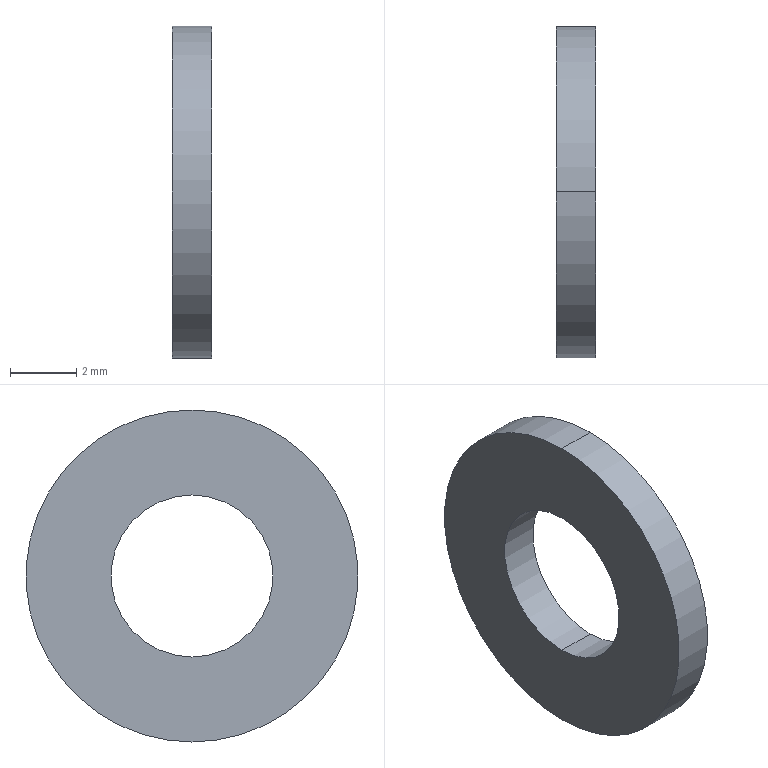Part | STEP file | flat washer narrow_am_B18.22M - Plain washer, 4 mm, narrow | 1 solid | 6 faces | box 1.2 x 10 x 10 mm | volume 71.803 mm3 | cylinder 4 | plane 2 | commonest cylinder face diameters 4.88 x2 10 x2
STEP:
#1=CARTESIAN_POINT('',(0.,0.,0.));
#2=DIRECTION('',(0.,0.,1.));
#3=DIRECTION('',(1.,0.,0.));
#4=AXIS2_PLACEMENT_3D('',#1,#2,#3);
#5=CARTESIAN_POINT('',(0.,0.,5.));
#6=VERTEX_POINT('',#5);
#7=CARTESIAN_POINT('',(0.,0.,-5.));
#8=VERTEX_POINT('',#7);
#9=CARTESIAN_POINT('',(0.,0.,0.));
#10=DIRECTION('',(-1.,0.,0.));
#11=DIRECTION('',(0.,0.,1.));
#12=AXIS2_PLACEMENT_3D('',#9,#10,#11);
#13=CIRCLE('',#12,5.);
#14=CARTESIAN_POINT('',(-34.925,0.,0.));
#15=DIRECTION('',(-1.,0.,0.));
#16=DIRECTION('',(0.,0.,1.));
#17=AXIS2_PLACEMENT_3D('',#14,#15,#16);
#18=CYLINDRICAL_SURFACE('',#17,5.);
#19=CARTESIAN_POINT('',(0.,-34.925));
#20=DIRECTION('',(1.,0.));
#21=VECTOR('',#20,1.);
#22=LINE('',#19,#21);
#23=(GEOMETRIC_REPRESENTATION_CONTEXT(2)PARAMETRIC_REPRESENTATION_CONTEXT()REPRESENTATION_CONTEXT('',''));
#24=DEFINITIONAL_REPRESENTATION('',(#22),#23);
#25=PCURVE('',#18,#24);
#26=CARTESIAN_POINT('',(0.,2.44,0.));
#27=DIRECTION('',(-1.,0.,0.));
#28=DIRECTION('',(0.,0.,1.));
#29=AXIS2_PLACEMENT_3D('',#26,#27,#28);
#30=PLANE('',#29);
#31=CARTESIAN_POINT('',(0.,-2.44));
#32=DIRECTION('',(1.,0.));
#33=AXIS2_PLACEMENT_2D('',#31,#32);
#34=CIRCLE('',#33,5.);
#35=(GEOMETRIC_REPRESENTATION_CONTEXT(2)PARAMETRIC_REPRESENTATION_CONTEXT()REPRESENTATION_CONTEXT('',''));
#36=DEFINITIONAL_REPRESENTATION('',(#34),#35);
#37=PCURVE('',#30,#36);
#38=SURFACE_CURVE('',#13,(#25,#37),.PCURVE_S1.);
#39=EDGE_CURVE('',#6,#8,#38,.T.);
#40=ORIENTED_EDGE('',*,*,#39,.T.);
#41=CARTESIAN_POINT('',(-1.2,0.,-5.));
#42=VERTEX_POINT('',#41);
#43=CARTESIAN_POINT('',(-34.925,0.,-5.));
#44=DIRECTION('',(-1.,0.,0.));
#45=VECTOR('',#44,1.);
#46=LINE('',#43,#45);
#47=CARTESIAN_POINT('',(3.142,0.));
#48=DIRECTION('',(0.,1.));
#49=VECTOR('',#48,1.);
#50=LINE('',#47,#49);
#51=(GEOMETRIC_REPRESENTATION_CONTEXT(2)PARAMETRIC_REPRESENTATION_CONTEXT()REPRESENTATION_CONTEXT('',''));
#52=DEFINITIONAL_REPRESENTATION('',(#50),#51);
#53=PCURVE('',#18,#52);
#54=CARTESIAN_POINT('',(-34.925,0.,0.));
#55=DIRECTION('',(-1.,0.,0.));
#56=DIRECTION('',(0.,0.,1.));
#57=AXIS2_PLACEMENT_3D('',#54,#55,#56);
#58=CYLINDRICAL_SURFACE('',#57,5.);
#59=CARTESIAN_POINT('',(3.142,0.));
#60=DIRECTION('',(0.,1.));
#61=VECTOR('',#60,1.);
#62=LINE('',#59,#61);
#63=(GEOMETRIC_REPRESENTATION_CONTEXT(2)PARAMETRIC_REPRESENTATION_CONTEXT()REPRESENTATION_CONTEXT('',''));
#64=DEFINITIONAL_REPRESENTATION('',(#62),#63);
#65=PCURVE('',#58,#64);
#66=SURFACE_CURVE('',#46,(#53,#65),.PCURVE_S1.);
#67=EDGE_CURVE('',#8,#42,#66,.T.);
#68=ORIENTED_EDGE('',*,*,#67,.T.);
#69=CARTESIAN_POINT('',(-1.2,0.,5.));
#70=VERTEX_POINT('',#69);
#71=CARTESIAN_POINT('',(-1.2,0.,0.));
#72=DIRECTION('',(-1.,0.,0.));
#73=DIRECTION('',(0.,0.,1.));
#74=AXIS2_PLACEMENT_3D('',#71,#72,#73);
#75=CIRCLE('',#74,5.);
#76=CARTESIAN_POINT('',(0.,-33.725));
#77=DIRECTION('',(1.,0.));
#78=VECTOR('',#77,1.);
#79=LINE('',#76,#78);
#80=(GEOMETRIC_REPRESENTATION_CONTEXT(2)PARAMETRIC_REPRESENTATION_CONTEXT()REPRESENTATION_CONTEXT('',''));
#81=DEFINITIONAL_REPRESENTATION('',(#79),#80);
#82=PCURVE('',#18,#81);
#83=CARTESIAN_POINT('',(-1.2,5.,0.));
#84=DIRECTION('',(1.,0.,0.));
#85=DIRECTION('',(0.,0.,-1.));
#86=AXIS2_PLACEMENT_3D('',#83,#84,#85);
#87=PLANE('',#86);
#88=CARTESIAN_POINT('',(-5.,-5.));
#89=CARTESIAN_POINT('',(-5.,3.66));
#90=CARTESIAN_POINT('',(2.5,-0.6699));
#91=CARTESIAN_POINT('',(10.,-5.));
#92=CARTESIAN_POINT('',(2.5,-9.33));
#93=CARTESIAN_POINT('',(-5.,-13.66));
#94=CARTESIAN_POINT('',(-5.,-5.));
#95=(BOUNDED_CURVE()B_SPLINE_CURVE(2,(#88,#89,#90,#91,#92,#93,#94),.UNSPECIFIED.,.T.,.F.)B_SPLINE_CURVE_WITH_KNOTS((1,2,2,2,2,1),(-2.094,0.,2.094,4.189,6.283,8.378),.UNSPECIFIED.)CURVE()GEOMETRIC_REPRESENTATION_ITEM()RATIONAL_B_SPLINE_CURVE((1.,0.5,1.,0.5,1.,0.5,1.))REPRESENTATION_ITEM(''));
#96=(GEOMETRIC_REPRESENTATION_CONTEXT(2)PARAMETRIC_REPRESENTATION_CONTEXT()REPRESENTATION_CONTEXT('',''));
#97=DEFINITIONAL_REPRESENTATION('',(#95),#96);
#98=PCURVE('',#87,#97);
#99=SURFACE_CURVE('',#75,(#82,#98),.PCURVE_S1.);
#100=EDGE_CURVE('',#70,#42,#99,.T.);
#101=ORIENTED_EDGE('',*,*,#100,.F.);
#102=CARTESIAN_POINT('',(-34.925,0.,5.));
#103=DIRECTION('',(-1.,0.,0.));
#104=VECTOR('',#103,1.);
#105=LINE('',#102,#104);
#106=CARTESIAN_POINT('',(0.,0.));
#107=DIRECTION('',(0.,1.));
#108=VECTOR('',#107,1.);
#109=LINE('',#106,#108);
#110=(GEOMETRIC_REPRESENTATION_CONTEXT(2)PARAMETRIC_REPRESENTATION_CONTEXT()REPRESENTATION_CONTEXT('',''));
#111=DEFINITIONAL_REPRESENTATION('',(#109),#110);
#112=PCURVE('',#18,#111);
#113=CARTESIAN_POINT('',(6.283,0.));
#114=DIRECTION('',(0.,1.));
#115=VECTOR('',#114,1.);
#116=LINE('',#113,#115);
#117=(GEOMETRIC_REPRESENTATION_CONTEXT(2)PARAMETRIC_REPRESENTATION_CONTEXT()REPRESENTATION_CONTEXT('',''));
#118=DEFINITIONAL_REPRESENTATION('',(#116),#117);
#119=PCURVE('',#58,#118);
#120=SURFACE_CURVE('',#105,(#112,#119),.PCURVE_S1.);
#121=EDGE_CURVE('',#6,#70,#120,.T.);
#122=ORIENTED_EDGE('',*,*,#121,.F.);
#123=EDGE_LOOP('',(#40,#68,#101,#122));
#124=FACE_BOUND('',#123,.T.);
#125=ADVANCED_FACE('',(#124),#18,.T.);
#126=CARTESIAN_POINT('',(0.,0.,2.44));
#127=VERTEX_POINT('',#126);
#128=CARTESIAN_POINT('',(-1.2,0.,2.44));
#129=VERTEX_POINT('',#128);
#130=CARTESIAN_POINT('',(-34.925,0.,2.44));
#131=DIRECTION('',(-1.,0.,0.));
#132=VECTOR('',#131,1.);
#133=LINE('',#130,#132);
#134=CARTESIAN_POINT('',(-34.925,0.,0.));
#135=DIRECTION('',(-1.,0.,0.));
#136=DIRECTION('',(0.,0.,1.));
#137=AXIS2_PLACEMENT_3D('',#134,#135,#136);
#138=CYLINDRICAL_SURFACE('',#137,2.44);
#139=CARTESIAN_POINT('',(6.283,0.));
#140=DIRECTION('',(0.,1.));
#141=VECTOR('',#140,1.);
#142=LINE('',#139,#141);
#143=(GEOMETRIC_REPRESENTATION_CONTEXT(2)PARAMETRIC_REPRESENTATION_CONTEXT()REPRESENTATION_CONTEXT('',''));
#144=DEFINITIONAL_REPRESENTATION('',(#142),#143);
#145=PCURVE('',#138,#144);
#146=CARTESIAN_POINT('',(-34.925,0.,0.));
#147=DIRECTION('',(-1.,0.,0.));
#148=DIRECTION('',(0.,0.,1.));
#149=AXIS2_PLACEMENT_3D('',#146,#147,#148);
#150=CYLINDRICAL_SURFACE('',#149,2.44);
#151=CARTESIAN_POINT('',(0.,0.));
#152=DIRECTION('',(0.,1.));
#153=VECTOR('',#152,1.);
#154=LINE('',#151,#153);
#155=(GEOMETRIC_REPRESENTATION_CONTEXT(2)PARAMETRIC_REPRESENTATION_CONTEXT()REPRESENTATION_CONTEXT('',''));
#156=DEFINITIONAL_REPRESENTATION('',(#154),#155);
#157=PCURVE('',#150,#156);
#158=SURFACE_CURVE('',#133,(#145,#157),.PCURVE_S1.);
#159=EDGE_CURVE('',#127,#129,#158,.T.);
#160=ORIENTED_EDGE('',*,*,#159,.T.);
#161=CARTESIAN_POINT('',(-1.2,0.,-2.44));
#162=VERTEX_POINT('',#161);
#163=CARTESIAN_POINT('',(-1.2,0.,0.));
#164=DIRECTION('',(-1.,0.,0.));
#165=DIRECTION('',(0.,0.,1.));
#166=AXIS2_PLACEMENT_3D('',#163,#164,#165);
#167=CIRCLE('',#166,2.44);
#168=CARTESIAN_POINT('',(0.,-33.725));
#169=DIRECTION('',(1.,0.));
#170=VECTOR('',#169,1.);
#171=LINE('',#168,#170);
#172=(GEOMETRIC_REPRESENTATION_CONTEXT(2)PARAMETRIC_REPRESENTATION_CONTEXT()REPRESENTATION_CONTEXT('',''));
#173=DEFINITIONAL_REPRESENTATION('',(#171),#172);
#174=PCURVE('',#138,#173);
#175=CARTESIAN_POINT('',(-2.44,-5.));
#176=CARTESIAN_POINT('',(-2.44,-0.7738));
#177=CARTESIAN_POINT('',(1.22,-2.887));
#178=CARTESIAN_POINT('',(4.88,-5.));
#179=CARTESIAN_POINT('',(1.22,-7.113));
#180=CARTESIAN_POINT('',(-2.44,-9.226));
#181=CARTESIAN_POINT('',(-2.44,-5.));
#182=(BOUNDED_CURVE()B_SPLINE_CURVE(2,(#175,#176,#177,#178,#179,#180,#181),.UNSPECIFIED.,.T.,.F.)B_SPLINE_CURVE_WITH_KNOTS((1,2,2,2,2,1),(-2.094,0.,2.094,4.189,6.283,8.378),.UNSPECIFIED.)CURVE()GEOMETRIC_REPRESENTATION_ITEM()RATIONAL_B_SPLINE_CURVE((1.,0.5,1.,0.5,1.,0.5,1.))REPRESENTATION_ITEM(''));
#183=(GEOMETRIC_REPRESENTATION_CONTEXT(2)PARAMETRIC_REPRESENTATION_CONTEXT()REPRESENTATION_CONTEXT('',''));
#184=DEFINITIONAL_REPRESENTATION('',(#182),#183);
#185=PCURVE('',#87,#184);
#186=SURFACE_CURVE('',#167,(#174,#185),.PCURVE_S1.);
#187=EDGE_CURVE('',#162,#129,#186,.T.);
#188=ORIENTED_EDGE('',*,*,#187,.F.);
#189=CARTESIAN_POINT('',(0.,0.,-2.44));
#190=VERTEX_POINT('',#189);
#191=CARTESIAN_POINT('',(-34.925,0.,-2.44));
#192=DIRECTION('',(-1.,0.,0.));
#193=VECTOR('',#192,1.);
#194=LINE('',#191,#193);
#195=CARTESIAN_POINT('',(3.142,0.));
#196=DIRECTION('',(0.,1.));
#197=VECTOR('',#196,1.);
#198=LINE('',#195,#197);
#199=(GEOMETRIC_REPRESENTATION_CONTEXT(2)PARAMETRIC_REPRESENTATION_CONTEXT()REPRESENTATION_CONTEXT('',''));
#200=DEFINITIONAL_REPRESENTATION('',(#198),#199);
#201=PCURVE('',#138,#200);
#202=CARTESIAN_POINT('',(3.142,0.));
#203=DIRECTION('',(0.,1.));
#204=VECTOR('',#203,1.);
#205=LINE('',#202,#204);
#206=(GEOMETRIC_REPRESENTATION_CONTEXT(2)PARAMETRIC_REPRESENTATION_CONTEXT()REPRESENTATION_CONTEXT('',''));
#207=DEFINITIONAL_REPRESENTATION('',(#205),#206);
#208=PCURVE('',#150,#207);
#209=SURFACE_CURVE('',#194,(#201,#208),.PCURVE_S1.);
#210=EDGE_CURVE('',#190,#162,#209,.T.);
#211=ORIENTED_EDGE('',*,*,#210,.F.);
#212=CARTESIAN_POINT('',(0.,0.,0.));
#213=DIRECTION('',(-1.,0.,0.));
#214=DIRECTION('',(0.,0.,1.));
#215=AXIS2_PLACEMENT_3D('',#212,#213,#214);
#216=CIRCLE('',#215,2.44);
#217=CARTESIAN_POINT('',(0.,-34.925));
#218=DIRECTION('',(1.,0.));
#219=VECTOR('',#218,1.);
#220=LINE('',#217,#219);
#221=(GEOMETRIC_REPRESENTATION_CONTEXT(2)PARAMETRIC_REPRESENTATION_CONTEXT()REPRESENTATION_CONTEXT('',''));
#222=DEFINITIONAL_REPRESENTATION('',(#220),#221);
#223=PCURVE('',#138,#222);
#224=CARTESIAN_POINT('',(0.,-2.44));
#225=DIRECTION('',(1.,0.));
#226=AXIS2_PLACEMENT_2D('',#224,#225);
#227=CIRCLE('',#226,2.44);
#228=(GEOMETRIC_REPRESENTATION_CONTEXT(2)PARAMETRIC_REPRESENTATION_CONTEXT()REPRESENTATION_CONTEXT('',''));
#229=DEFINITIONAL_REPRESENTATION('',(#227),#228);
#230=PCURVE('',#30,#229);
#231=SURFACE_CURVE('',#216,(#223,#230),.PCURVE_S1.);
#232=EDGE_CURVE('',#190,#127,#231,.T.);
#233=ORIENTED_EDGE('',*,*,#232,.T.);
#234=EDGE_LOOP('',(#160,#188,#211,#233));
#235=FACE_BOUND('',#234,.F.);
#236=ADVANCED_FACE('',(#235),#138,.F.);
#237=CARTESIAN_POINT('',(-1.2,0.,0.));
#238=DIRECTION('',(-1.,0.,0.));
#239=DIRECTION('',(0.,0.,1.));
#240=AXIS2_PLACEMENT_3D('',#237,#238,#239);
#241=CIRCLE('',#240,2.44);
#242=CARTESIAN_POINT('',(0.,-33.725));
#243=DIRECTION('',(1.,0.));
#244=VECTOR('',#243,1.);
#245=LINE('',#242,#244);
#246=(GEOMETRIC_REPRESENTATION_CONTEXT(2)PARAMETRIC_REPRESENTATION_CONTEXT()REPRESENTATION_CONTEXT('',''));
#247=DEFINITIONAL_REPRESENTATION('',(#245),#246);
#248=PCURVE('',#150,#247);
#249=CARTESIAN_POINT('',(-2.44,-5.));
#250=CARTESIAN_POINT('',(-2.44,-0.7738));
#251=CARTESIAN_POINT('',(1.22,-2.887));
#252=CARTESIAN_POINT('',(4.88,-5.));
#253=CARTESIAN_POINT('',(1.22,-7.113));
#254=CARTESIAN_POINT('',(-2.44,-9.226));
#255=CARTESIAN_POINT('',(-2.44,-5.));
#256=(BOUNDED_CURVE()B_SPLINE_CURVE(2,(#249,#250,#251,#252,#253,#254,#255),.UNSPECIFIED.,.T.,.F.)B_SPLINE_CURVE_WITH_KNOTS((1,2,2,2,2,1),(-2.094,0.,2.094,4.189,6.283,8.378),.UNSPECIFIED.)CURVE()GEOMETRIC_REPRESENTATION_ITEM()RATIONAL_B_SPLINE_CURVE((1.,0.5,1.,0.5,1.,0.5,1.))REPRESENTATION_ITEM(''));
#257=(GEOMETRIC_REPRESENTATION_CONTEXT(2)PARAMETRIC_REPRESENTATION_CONTEXT()REPRESENTATION_CONTEXT('',''));
#258=DEFINITIONAL_REPRESENTATION('',(#256),#257);
#259=PCURVE('',#87,#258);
#260=SURFACE_CURVE('',#241,(#248,#259),.PCURVE_S1.);
#261=EDGE_CURVE('',#129,#162,#260,.T.);
#262=ORIENTED_EDGE('',*,*,#261,.F.);
#263=ORIENTED_EDGE('',*,*,#159,.F.);
#264=CARTESIAN_POINT('',(0.,0.,0.));
#265=DIRECTION('',(-1.,0.,0.));
#266=DIRECTION('',(0.,0.,1.));
#267=AXIS2_PLACEMENT_3D('',#264,#265,#266);
#268=CIRCLE('',#267,2.44);
#269=CARTESIAN_POINT('',(0.,-34.925));
#270=DIRECTION('',(1.,0.));
#271=VECTOR('',#270,1.);
#272=LINE('',#269,#271);
#273=(GEOMETRIC_REPRESENTATION_CONTEXT(2)PARAMETRIC_REPRESENTATION_CONTEXT()REPRESENTATION_CONTEXT('',''));
#274=DEFINITIONAL_REPRESENTATION('',(#272),#273);
#275=PCURVE('',#150,#274);
#276=CARTESIAN_POINT('',(0.,-2.44));
#277=DIRECTION('',(1.,0.));
#278=AXIS2_PLACEMENT_2D('',#276,#277);
#279=CIRCLE('',#278,2.44);
#280=(GEOMETRIC_REPRESENTATION_CONTEXT(2)PARAMETRIC_REPRESENTATION_CONTEXT()REPRESENTATION_CONTEXT('',''));
#281=DEFINITIONAL_REPRESENTATION('',(#279),#280);
#282=PCURVE('',#30,#281);
#283=SURFACE_CURVE('',#268,(#275,#282),.PCURVE_S1.);
#284=EDGE_CURVE('',#127,#190,#283,.T.);
#285=ORIENTED_EDGE('',*,*,#284,.T.);
#286=ORIENTED_EDGE('',*,*,#210,.T.);
#287=EDGE_LOOP('',(#262,#263,#285,#286));
#288=FACE_BOUND('',#287,.F.);
#289=ADVANCED_FACE('',(#288),#150,.F.);
#290=ORIENTED_EDGE('',*,*,#39,.F.);
#291=CARTESIAN_POINT('',(0.,0.,0.));
#292=DIRECTION('',(-1.,0.,0.));
#293=DIRECTION('',(0.,0.,1.));
#294=AXIS2_PLACEMENT_3D('',#291,#292,#293);
#295=CIRCLE('',#294,5.);
#296=CARTESIAN_POINT('',(0.,-2.44));
#297=DIRECTION('',(1.,0.));
#298=AXIS2_PLACEMENT_2D('',#296,#297);
#299=CIRCLE('',#298,5.);
#300=(GEOMETRIC_REPRESENTATION_CONTEXT(2)PARAMETRIC_REPRESENTATION_CONTEXT()REPRESENTATION_CONTEXT('',''));
#301=DEFINITIONAL_REPRESENTATION('',(#299),#300);
#302=PCURVE('',#30,#301);
#303=CARTESIAN_POINT('',(0.,-34.925));
#304=DIRECTION('',(1.,0.));
#305=VECTOR('',#304,1.);
#306=LINE('',#303,#305);
#307=(GEOMETRIC_REPRESENTATION_CONTEXT(2)PARAMETRIC_REPRESENTATION_CONTEXT()REPRESENTATION_CONTEXT('',''));
#308=DEFINITIONAL_REPRESENTATION('',(#306),#307);
#309=PCURVE('',#58,#308);
#310=SURFACE_CURVE('',#295,(#302,#309),.PCURVE_S1.);
#311=EDGE_CURVE('',#8,#6,#310,.T.);
#312=ORIENTED_EDGE('',*,*,#311,.F.);
#313=EDGE_LOOP('',(#290,#312));
#314=FACE_BOUND('',#313,.T.);
#315=ORIENTED_EDGE('',*,*,#284,.T.);
#316=ORIENTED_EDGE('',*,*,#232,.T.);
#317=EDGE_LOOP('',(#315,#316));
#318=FACE_BOUND('',#317,.T.);
#319=ADVANCED_FACE('',(#314,#318),#30,.F.);
#320=ORIENTED_EDGE('',*,*,#67,.F.);
#321=ORIENTED_EDGE('',*,*,#311,.T.);
#322=ORIENTED_EDGE('',*,*,#121,.T.);
#323=CARTESIAN_POINT('',(-1.2,0.,0.));
#324=DIRECTION('',(-1.,0.,0.));
#325=DIRECTION('',(0.,0.,1.));
#326=AXIS2_PLACEMENT_3D('',#323,#324,#325);
#327=CIRCLE('',#326,5.);
#328=CARTESIAN_POINT('',(0.,-33.725));
#329=DIRECTION('',(1.,0.));
#330=VECTOR('',#329,1.);
#331=LINE('',#328,#330);
#332=(GEOMETRIC_REPRESENTATION_CONTEXT(2)PARAMETRIC_REPRESENTATION_CONTEXT()REPRESENTATION_CONTEXT('',''));
#333=DEFINITIONAL_REPRESENTATION('',(#331),#332);
#334=PCURVE('',#58,#333);
#335=CARTESIAN_POINT('',(-5.,-5.));
#336=CARTESIAN_POINT('',(-5.,3.66));
#337=CARTESIAN_POINT('',(2.5,-0.6699));
#338=CARTESIAN_POINT('',(10.,-5.));
#339=CARTESIAN_POINT('',(2.5,-9.33));
#340=CARTESIAN_POINT('',(-5.,-13.66));
#341=CARTESIAN_POINT('',(-5.,-5.));
#342=(BOUNDED_CURVE()B_SPLINE_CURVE(2,(#335,#336,#337,#338,#339,#340,#341),.UNSPECIFIED.,.T.,.F.)B_SPLINE_CURVE_WITH_KNOTS((1,2,2,2,2,1),(-2.094,0.,2.094,4.189,6.283,8.378),.UNSPECIFIED.)CURVE()GEOMETRIC_REPRESENTATION_ITEM()RATIONAL_B_SPLINE_CURVE((1.,0.5,1.,0.5,1.,0.5,1.))REPRESENTATION_ITEM(''));
#343=(GEOMETRIC_REPRESENTATION_CONTEXT(2)PARAMETRIC_REPRESENTATION_CONTEXT()REPRESENTATION_CONTEXT('',''));
#344=DEFINITIONAL_REPRESENTATION('',(#342),#343);
#345=PCURVE('',#87,#344);
#346=SURFACE_CURVE('',#327,(#334,#345),.PCURVE_S1.);
#347=EDGE_CURVE('',#42,#70,#346,.T.);
#348=ORIENTED_EDGE('',*,*,#347,.F.);
#349=EDGE_LOOP('',(#320,#321,#322,#348));
#350=FACE_BOUND('',#349,.T.);
#351=ADVANCED_FACE('',(#350),#58,.T.);
#352=ORIENTED_EDGE('',*,*,#261,.F.);
#353=ORIENTED_EDGE('',*,*,#187,.F.);
#354=EDGE_LOOP('',(#352,#353));
#355=FACE_BOUND('',#354,.T.);
#356=ORIENTED_EDGE('',*,*,#100,.T.);
#357=ORIENTED_EDGE('',*,*,#347,.T.);
#358=EDGE_LOOP('',(#356,#357));
#359=FACE_BOUND('',#358,.T.);
#360=ADVANCED_FACE('',(#355,#359),#87,.F.);
#361=CLOSED_SHELL('',(#125,#236,#289,#319,#351,#360));
#362=MANIFOLD_SOLID_BREP('',#361);
#363=(LENGTH_UNIT()NAMED_UNIT(*)SI_UNIT(.MILLI.,.METRE.));
#364=UNCERTAINTY_MEASURE_WITH_UNIT(LENGTH_MEASURE(0.0000001),#363,'','');
#365=(NAMED_UNIT(*)PLANE_ANGLE_UNIT()SI_UNIT($,.RADIAN.));
#366=(NAMED_UNIT(*)SI_UNIT($,.STERADIAN.)SOLID_ANGLE_UNIT());
#367=(GEOMETRIC_REPRESENTATION_CONTEXT(3)GLOBAL_UNCERTAINTY_ASSIGNED_CONTEXT((#364))GLOBAL_UNIT_ASSIGNED_CONTEXT((#363,#365,#366))REPRESENTATION_CONTEXT('',''));
#368=ADVANCED_BREP_SHAPE_REPRESENTATION('',(#4,#362),#367);